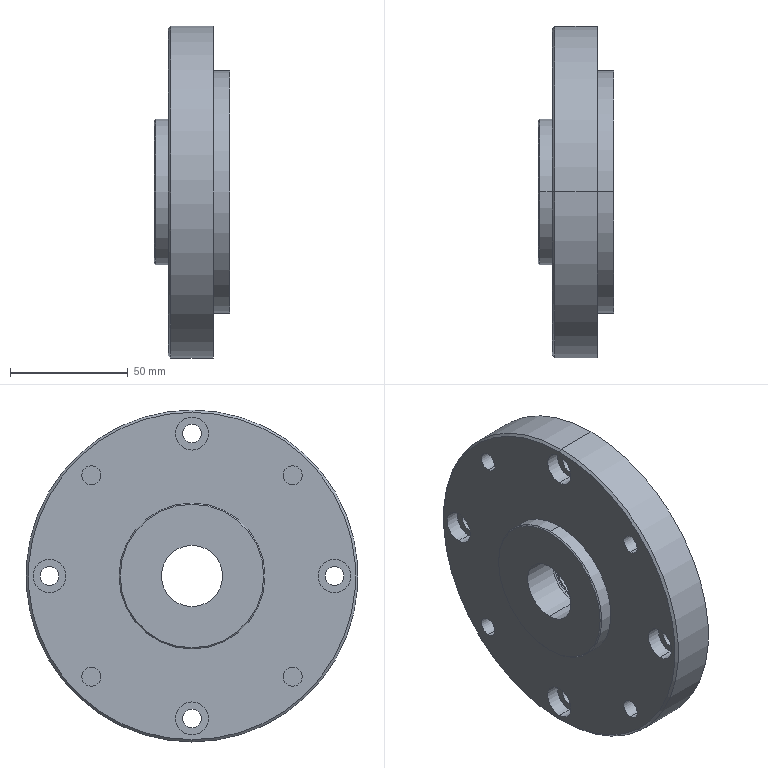Part | SolidWorks | features ICE 3, Chamfer 2, Revolution 2 | 2 solids | 58 faces | box 32 x 141 x 141 mm | volume 347487 mm3 | cylinder 36 | plane 14 | torus 4 | cone 4 | commonest cylinder face diameters 8 x16 14 x8 26 x4 30 x2 62 x2 103 x2